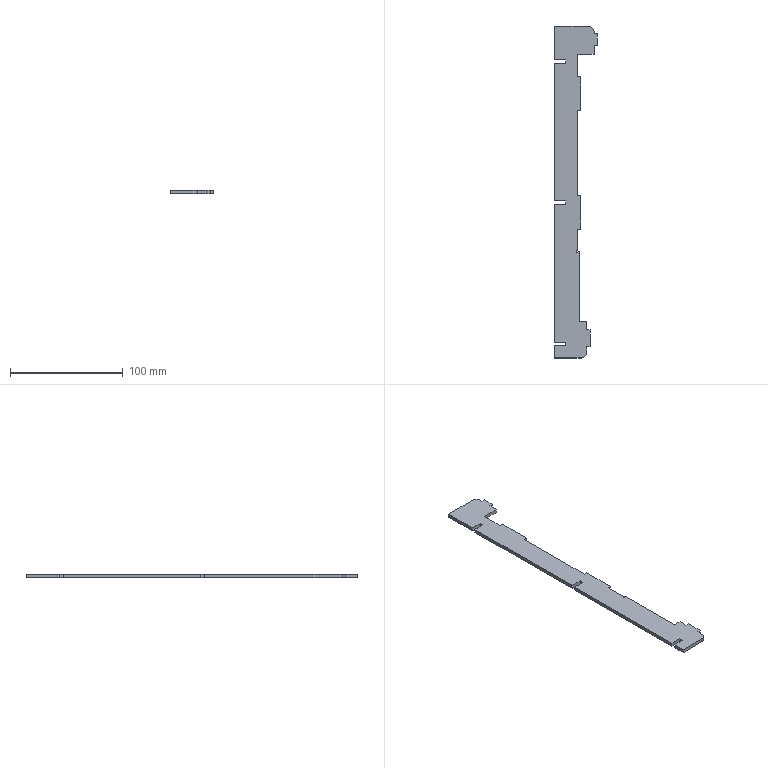Part | SolidWorks | features FlatPattern 1, SMBaseFlange 1, SheetMetal 1 | 1 solid | 46 faces | box 38 x 294.081 x 3.2 mm | volume 21708 mm3 | plane 40 | cylinder 6 | commonest cylinder face diameters 1 x2 1.5 x2 10 x2
STEP:
#1=CARTESIAN_POINT('',(397.65,-115.276,3.2));
#2=VERTEX_POINT('',#1);
#3=CARTESIAN_POINT('',(398.1,-114.588,3.2));
#4=VERTEX_POINT('',#3);
#5=CARTESIAN_POINT('',(398.4,-115.276,3.2));
#6=DIRECTION('',(0.,0.,-1.));
#7=DIRECTION('',(1.,0.,0.));
#8=AXIS2_PLACEMENT_3D('',#5,#6,#7);
#9=CIRCLE('',#8,0.75);
#10=EDGE_CURVE('',#2,#4,#9,.T.);
#11=ORIENTED_EDGE('',*,*,#10,.F.);
#12=CARTESIAN_POINT('',(397.65,-115.276,0.));
#13=VERTEX_POINT('',#12);
#14=CARTESIAN_POINT('',(397.65,-115.276,3.2));
#15=DIRECTION('',(0.,0.,-1.));
#16=VECTOR('',#15,1000.);
#17=LINE('',#14,#16);
#18=EDGE_CURVE('',#2,#13,#17,.T.);
#19=ORIENTED_EDGE('',*,*,#18,.T.);
#20=CARTESIAN_POINT('',(398.1,-114.588,0.));
#21=VERTEX_POINT('',#20);
#22=CARTESIAN_POINT('',(398.4,-115.276,0.));
#23=DIRECTION('',(0.,0.,-1.));
#24=DIRECTION('',(1.,0.,0.));
#25=AXIS2_PLACEMENT_3D('',#22,#23,#24);
#26=CIRCLE('',#25,0.75);
#27=EDGE_CURVE('',#13,#21,#26,.T.);
#28=ORIENTED_EDGE('',*,*,#27,.T.);
#29=CARTESIAN_POINT('',(398.1,-114.588,3.2));
#30=DIRECTION('',(0.,0.,-1.));
#31=VECTOR('',#30,1000.);
#32=LINE('',#29,#31);
#33=EDGE_CURVE('',#4,#21,#32,.T.);
#34=ORIENTED_EDGE('',*,*,#33,.F.);
#35=EDGE_LOOP('',(#11,#19,#28,#34));
#36=FACE_OUTER_BOUND('',#35,.T.);
#37=CARTESIAN_POINT('',(398.4,-115.276,3.2));
#38=DIRECTION('',(0.,0.,-1.));
#39=DIRECTION('',(-1.,0.,0.));
#40=AXIS2_PLACEMENT_3D('',#37,#38,#39);
#41=CYLINDRICAL_SURFACE('',#40,0.75);
#42=ADVANCED_FACE('',(#36),#41,.F.);
#43=CARTESIAN_POINT('',(413.4,59.724,0.));
#44=VERTEX_POINT('',#43);
#45=CARTESIAN_POINT('',(413.4,67.724,0.));
#46=VERTEX_POINT('',#45);
#47=CARTESIAN_POINT('',(413.4,59.724,0.));
#48=DIRECTION('',(0.,1.,0.));
#49=VECTOR('',#48,1000.);
#50=LINE('',#47,#49);
#51=EDGE_CURVE('',#44,#46,#50,.T.);
#52=ORIENTED_EDGE('',*,*,#51,.T.);
#53=CARTESIAN_POINT('',(413.4,67.724,3.2));
#54=VERTEX_POINT('',#53);
#55=CARTESIAN_POINT('',(413.4,67.724,3.2));
#56=DIRECTION('',(0.,0.,-1.));
#57=VECTOR('',#56,1000.);
#58=LINE('',#55,#57);
#59=EDGE_CURVE('',#54,#46,#58,.T.);
#60=ORIENTED_EDGE('',*,*,#59,.F.);
#61=CARTESIAN_POINT('',(413.4,59.724,3.2));
#62=VERTEX_POINT('',#61);
#63=CARTESIAN_POINT('',(413.4,59.724,3.2));
#64=DIRECTION('',(0.,1.,0.));
#65=VECTOR('',#64,1000.);
#66=LINE('',#63,#65);
#67=EDGE_CURVE('',#62,#54,#66,.T.);
#68=ORIENTED_EDGE('',*,*,#67,.F.);
#69=CARTESIAN_POINT('',(413.4,59.724,3.2));
#70=DIRECTION('',(0.,0.,-1.));
#71=VECTOR('',#70,1000.);
#72=LINE('',#69,#71);
#73=EDGE_CURVE('',#62,#44,#72,.T.);
#74=ORIENTED_EDGE('',*,*,#73,.T.);
#75=EDGE_LOOP('',(#52,#60,#68,#74));
#76=FACE_OUTER_BOUND('',#75,.T.);
#77=CARTESIAN_POINT('',(413.4,59.724,3.2));
#78=DIRECTION('',(-1.,0.,0.));
#79=DIRECTION('',(0.,-1.,0.));
#80=AXIS2_PLACEMENT_3D('',#77,#78,#79);
#81=PLANE('',#80);
#82=ADVANCED_FACE('',(#76),#81,.F.);
#83=CARTESIAN_POINT('',(416.4,67.724,0.));
#84=VERTEX_POINT('',#83);
#85=CARTESIAN_POINT('',(416.4,67.724,0.));
#86=DIRECTION('',(1.,0.,0.));
#87=VECTOR('',#86,1000.);
#88=LINE('',#85,#87);
#89=EDGE_CURVE('',#46,#84,#88,.T.);
#90=ORIENTED_EDGE('',*,*,#89,.T.);
#91=CARTESIAN_POINT('',(416.4,67.724,3.2));
#92=VERTEX_POINT('',#91);
#93=CARTESIAN_POINT('',(416.4,67.724,3.2));
#94=DIRECTION('',(0.,0.,-1.));
#95=VECTOR('',#94,1000.);
#96=LINE('',#93,#95);
#97=EDGE_CURVE('',#92,#84,#96,.T.);
#98=ORIENTED_EDGE('',*,*,#97,.F.);
#99=CARTESIAN_POINT('',(416.4,67.724,3.2));
#100=DIRECTION('',(1.,0.,0.));
#101=VECTOR('',#100,1000.);
#102=LINE('',#99,#101);
#103=EDGE_CURVE('',#54,#92,#102,.T.);
#104=ORIENTED_EDGE('',*,*,#103,.F.);
#105=ORIENTED_EDGE('',*,*,#59,.T.);
#106=EDGE_LOOP('',(#90,#98,#104,#105));
#107=FACE_OUTER_BOUND('',#106,.T.);
#108=CARTESIAN_POINT('',(416.4,67.724,3.2));
#109=DIRECTION('',(0.,1.,0.));
#110=DIRECTION('',(0.,0.,1.));
#111=AXIS2_PLACEMENT_3D('',#108,#109,#110);
#112=PLANE('',#111);
#113=ADVANCED_FACE('',(#107),#112,.F.);
#114=CARTESIAN_POINT('',(416.4,77.724,0.));
#115=VERTEX_POINT('',#114);
#116=CARTESIAN_POINT('',(416.4,77.724,0.));
#117=DIRECTION('',(0.,1.,0.));
#118=VECTOR('',#117,1000.);
#119=LINE('',#116,#118);
#120=EDGE_CURVE('',#84,#115,#119,.T.);
#121=ORIENTED_EDGE('',*,*,#120,.T.);
#122=CARTESIAN_POINT('',(416.4,77.724,3.2));
#123=VERTEX_POINT('',#122);
#124=CARTESIAN_POINT('',(416.4,77.724,3.2));
#125=DIRECTION('',(0.,0.,-1.));
#126=VECTOR('',#125,1000.);
#127=LINE('',#124,#126);
#128=EDGE_CURVE('',#123,#115,#127,.T.);
#129=ORIENTED_EDGE('',*,*,#128,.F.);
#130=CARTESIAN_POINT('',(416.4,77.724,3.2));
#131=DIRECTION('',(0.,1.,0.));
#132=VECTOR('',#131,1000.);
#133=LINE('',#130,#132);
#134=EDGE_CURVE('',#92,#123,#133,.T.);
#135=ORIENTED_EDGE('',*,*,#134,.F.);
#136=ORIENTED_EDGE('',*,*,#97,.T.);
#137=EDGE_LOOP('',(#121,#129,#135,#136));
#138=FACE_OUTER_BOUND('',#137,.T.);
#139=CARTESIAN_POINT('',(416.4,77.724,3.2));
#140=DIRECTION('',(-1.,0.,0.));
#141=DIRECTION('',(0.,0.,1.));
#142=AXIS2_PLACEMENT_3D('',#139,#140,#141);
#143=PLANE('',#142);
#144=ADVANCED_FACE('',(#138),#143,.F.);
#145=CARTESIAN_POINT('',(413.4,77.724,0.));
#146=VERTEX_POINT('',#145);
#147=CARTESIAN_POINT('',(413.4,77.724,0.));
#148=DIRECTION('',(-1.,0.,0.));
#149=VECTOR('',#148,1000.);
#150=LINE('',#147,#149);
#151=EDGE_CURVE('',#115,#146,#150,.T.);
#152=ORIENTED_EDGE('',*,*,#151,.T.);
#153=CARTESIAN_POINT('',(413.4,77.724,3.2));
#154=VERTEX_POINT('',#153);
#155=CARTESIAN_POINT('',(413.4,77.724,3.2));
#156=DIRECTION('',(0.,0.,-1.));
#157=VECTOR('',#156,1000.);
#158=LINE('',#155,#157);
#159=EDGE_CURVE('',#154,#146,#158,.T.);
#160=ORIENTED_EDGE('',*,*,#159,.F.);
#161=CARTESIAN_POINT('',(413.4,77.724,3.2));
#162=DIRECTION('',(-1.,0.,0.));
#163=VECTOR('',#162,1000.);
#164=LINE('',#161,#163);
#165=EDGE_CURVE('',#123,#154,#164,.T.);
#166=ORIENTED_EDGE('',*,*,#165,.F.);
#167=ORIENTED_EDGE('',*,*,#128,.T.);
#168=EDGE_LOOP('',(#152,#160,#166,#167));
#169=FACE_OUTER_BOUND('',#168,.T.);
#170=CARTESIAN_POINT('',(413.4,77.724,3.2));
#171=DIRECTION('',(0.,-1.,0.));
#172=DIRECTION('',(0.,0.,-1.));
#173=AXIS2_PLACEMENT_3D('',#170,#171,#172);
#174=PLANE('',#173);
#175=ADVANCED_FACE('',(#169),#174,.F.);
#176=CARTESIAN_POINT('',(413.4,79.724,0.));
#177=VERTEX_POINT('',#176);
#178=CARTESIAN_POINT('',(413.4,77.724,0.));
#179=DIRECTION('',(0.,1.,0.));
#180=VECTOR('',#179,1000.);
#181=LINE('',#178,#180);
#182=EDGE_CURVE('',#146,#177,#181,.T.);
#183=ORIENTED_EDGE('',*,*,#182,.T.);
#184=CARTESIAN_POINT('',(413.4,79.724,3.2));
#185=VERTEX_POINT('',#184);
#186=CARTESIAN_POINT('',(413.4,79.724,3.2));
#187=DIRECTION('',(0.,0.,-1.));
#188=VECTOR('',#187,1000.);
#189=LINE('',#186,#188);
#190=EDGE_CURVE('',#185,#177,#189,.T.);
#191=ORIENTED_EDGE('',*,*,#190,.F.);
#192=CARTESIAN_POINT('',(413.4,77.724,3.2));
#193=DIRECTION('',(0.,1.,0.));
#194=VECTOR('',#193,1000.);
#195=LINE('',#192,#194);
#196=EDGE_CURVE('',#154,#185,#195,.T.);
#197=ORIENTED_EDGE('',*,*,#196,.F.);
#198=ORIENTED_EDGE('',*,*,#159,.T.);
#199=EDGE_LOOP('',(#183,#191,#197,#198));
#200=FACE_OUTER_BOUND('',#199,.T.);
#201=CARTESIAN_POINT('',(413.4,77.724,3.2));
#202=DIRECTION('',(-1.,0.,0.));
#203=DIRECTION('',(0.,0.,1.));
#204=AXIS2_PLACEMENT_3D('',#201,#202,#203);
#205=PLANE('',#204);
#206=ADVANCED_FACE('',(#200),#205,.F.);
#207=CARTESIAN_POINT('',(408.4,84.724,0.));
#208=VERTEX_POINT('',#207);
#209=CARTESIAN_POINT('',(408.4,79.724,0.));
#210=DIRECTION('',(0.,0.,1.));
#211=DIRECTION('',(1.,0.,0.));
#212=AXIS2_PLACEMENT_3D('',#209,#210,#211);
#213=CIRCLE('',#212,5.);
#214=EDGE_CURVE('',#177,#208,#213,.T.);
#215=ORIENTED_EDGE('',*,*,#214,.T.);
#216=CARTESIAN_POINT('',(408.4,84.724,3.2));
#217=VERTEX_POINT('',#216);
#218=CARTESIAN_POINT('',(408.4,84.724,3.2));
#219=DIRECTION('',(0.,0.,-1.));
#220=VECTOR('',#219,1000.);
#221=LINE('',#218,#220);
#222=EDGE_CURVE('',#217,#208,#221,.T.);
#223=ORIENTED_EDGE('',*,*,#222,.F.);
#224=CARTESIAN_POINT('',(408.4,79.724,3.2));
#225=DIRECTION('',(0.,0.,1.));
#226=DIRECTION('',(1.,0.,0.));
#227=AXIS2_PLACEMENT_3D('',#224,#225,#226);
#228=CIRCLE('',#227,5.);
#229=EDGE_CURVE('',#185,#217,#228,.T.);
#230=ORIENTED_EDGE('',*,*,#229,.F.);
#231=ORIENTED_EDGE('',*,*,#190,.T.);
#232=EDGE_LOOP('',(#215,#223,#230,#231));
#233=FACE_OUTER_BOUND('',#232,.T.);
#234=CARTESIAN_POINT('',(408.4,79.724,3.2));
#235=DIRECTION('',(0.,0.,-1.));
#236=DIRECTION('',(-1.,0.,0.));
#237=AXIS2_PLACEMENT_3D('',#234,#235,#236);
#238=CYLINDRICAL_SURFACE('',#237,5.);
#239=ADVANCED_FACE('',(#233),#238,.T.);
#240=CARTESIAN_POINT('',(378.4,84.724,0.));
#241=VERTEX_POINT('',#240);
#242=CARTESIAN_POINT('',(408.4,84.724,0.));
#243=DIRECTION('',(-1.,0.,0.));
#244=VECTOR('',#243,1000.);
#245=LINE('',#242,#244);
#246=EDGE_CURVE('',#208,#241,#245,.T.);
#247=ORIENTED_EDGE('',*,*,#246,.T.);
#248=CARTESIAN_POINT('',(378.4,84.724,3.2));
#249=VERTEX_POINT('',#248);
#250=CARTESIAN_POINT('',(378.4,84.724,3.2));
#251=DIRECTION('',(0.,0.,-1.));
#252=VECTOR('',#251,1000.);
#253=LINE('',#250,#252);
#254=EDGE_CURVE('',#249,#241,#253,.T.);
#255=ORIENTED_EDGE('',*,*,#254,.F.);
#256=CARTESIAN_POINT('',(408.4,84.724,3.2));
#257=DIRECTION('',(-1.,0.,0.));
#258=VECTOR('',#257,1000.);
#259=LINE('',#256,#258);
#260=EDGE_CURVE('',#217,#249,#259,.T.);
#261=ORIENTED_EDGE('',*,*,#260,.F.);
#262=ORIENTED_EDGE('',*,*,#222,.T.);
#263=EDGE_LOOP('',(#247,#255,#261,#262));
#264=FACE_OUTER_BOUND('',#263,.T.);
#265=CARTESIAN_POINT('',(408.4,84.724,3.2));
#266=DIRECTION('',(0.,-1.,0.));
#267=DIRECTION('',(0.,0.,-1.));
#268=AXIS2_PLACEMENT_3D('',#265,#266,#267);
#269=PLANE('',#268);
#270=ADVANCED_FACE('',(#264),#269,.F.);
#271=CARTESIAN_POINT('',(378.4,54.724,0.));
#272=VERTEX_POINT('',#271);
#273=CARTESIAN_POINT('',(378.4,84.724,0.));
#274=DIRECTION('',(0.,-1.,0.));
#275=VECTOR('',#274,1000.);
#276=LINE('',#273,#275);
#277=EDGE_CURVE('',#241,#272,#276,.T.);
#278=ORIENTED_EDGE('',*,*,#277,.T.);
#279=CARTESIAN_POINT('',(378.4,54.724,3.2));
#280=VERTEX_POINT('',#279);
#281=CARTESIAN_POINT('',(378.4,54.724,3.2));
#282=DIRECTION('',(0.,0.,-1.));
#283=VECTOR('',#282,1000.);
#284=LINE('',#281,#283);
#285=EDGE_CURVE('',#280,#272,#284,.T.);
#286=ORIENTED_EDGE('',*,*,#285,.F.);
#287=CARTESIAN_POINT('',(378.4,84.724,3.2));
#288=DIRECTION('',(0.,-1.,0.));
#289=VECTOR('',#288,1000.);
#290=LINE('',#287,#289);
#291=EDGE_CURVE('',#249,#280,#290,.T.);
#292=ORIENTED_EDGE('',*,*,#291,.F.);
#293=ORIENTED_EDGE('',*,*,#254,.T.);
#294=EDGE_LOOP('',(#278,#286,#292,#293));
#295=FACE_OUTER_BOUND('',#294,.T.);
#296=CARTESIAN_POINT('',(378.4,84.724,3.2));
#297=DIRECTION('',(1.,0.,0.));
#298=DIRECTION('',(0.,0.,-1.));
#299=AXIS2_PLACEMENT_3D('',#296,#297,#298);
#300=PLANE('',#299);
#301=ADVANCED_FACE('',(#295),#300,.F.);
#302=CARTESIAN_POINT('',(388.4,54.724,0.));
#303=VERTEX_POINT('',#302);
#304=CARTESIAN_POINT('',(378.4,54.724,0.));
#305=DIRECTION('',(1.,0.000000036,0.));
#306=VECTOR('',#305,1000.);
#307=LINE('',#304,#306);
#308=EDGE_CURVE('',#272,#303,#307,.T.);
#309=ORIENTED_EDGE('',*,*,#308,.T.);
#310=CARTESIAN_POINT('',(388.4,54.724,3.2));
#311=VERTEX_POINT('',#310);
#312=CARTESIAN_POINT('',(388.4,54.724,3.2));
#313=DIRECTION('',(0.,0.,-1.));
#314=VECTOR('',#313,1000.);
#315=LINE('',#312,#314);
#316=EDGE_CURVE('',#311,#303,#315,.T.);
#317=ORIENTED_EDGE('',*,*,#316,.F.);
#318=CARTESIAN_POINT('',(378.4,54.724,3.2));
#319=DIRECTION('',(1.,0.000000036,0.));
#320=VECTOR('',#319,1000.);
#321=LINE('',#318,#320);
#322=EDGE_CURVE('',#280,#311,#321,.T.);
#323=ORIENTED_EDGE('',*,*,#322,.F.);
#324=ORIENTED_EDGE('',*,*,#285,.T.);
#325=EDGE_LOOP('',(#309,#317,#323,#324));
#326=FACE_OUTER_BOUND('',#325,.T.);
#327=CARTESIAN_POINT('',(378.4,54.724,3.2));
#328=DIRECTION('',(-0.000000036,1.,0.));
#329=DIRECTION('',(-1.,-0.000000036,0.));
#330=AXIS2_PLACEMENT_3D('',#327,#328,#329);
#331=PLANE('',#330);
#332=ADVANCED_FACE('',(#326),#331,.F.);
#333=CARTESIAN_POINT('',(388.4,51.524,0.));
#334=VERTEX_POINT('',#333);
#335=CARTESIAN_POINT('',(388.4,54.724,0.));
#336=DIRECTION('',(0.000000036,-1.,0.));
#337=VECTOR('',#336,1000.);
#338=LINE('',#335,#337);
#339=EDGE_CURVE('',#303,#334,#338,.T.);
#340=ORIENTED_EDGE('',*,*,#339,.T.);
#341=CARTESIAN_POINT('',(388.4,51.524,3.2));
#342=VERTEX_POINT('',#341);
#343=CARTESIAN_POINT('',(388.4,51.524,3.2));
#344=DIRECTION('',(0.,0.,-1.));
#345=VECTOR('',#344,1000.);
#346=LINE('',#343,#345);
#347=EDGE_CURVE('',#342,#334,#346,.T.);
#348=ORIENTED_EDGE('',*,*,#347,.F.);
#349=CARTESIAN_POINT('',(388.4,54.724,3.2));
#350=DIRECTION('',(0.000000036,-1.,0.));
#351=VECTOR('',#350,1000.);
#352=LINE('',#349,#351);
#353=EDGE_CURVE('',#311,#342,#352,.T.);
#354=ORIENTED_EDGE('',*,*,#353,.F.);
#355=ORIENTED_EDGE('',*,*,#316,.T.);
#356=EDGE_LOOP('',(#340,#348,#354,#355));
#357=FACE_OUTER_BOUND('',#356,.T.);
#358=CARTESIAN_POINT('',(388.4,54.724,3.2));
#359=DIRECTION('',(1.,0.000000036,0.));
#360=DIRECTION('',(-0.000000036,1.,0.));
#361=AXIS2_PLACEMENT_3D('',#358,#359,#360);
#362=PLANE('',#361);
#363=ADVANCED_FACE('',(#357),#362,.F.);
#364=CARTESIAN_POINT('',(378.4,51.524,0.));
#365=VERTEX_POINT('',#364);
#366=CARTESIAN_POINT('',(388.4,51.524,0.));
#367=DIRECTION('',(-1.,-0.000000036,0.));
#368=VECTOR('',#367,1000.);
#369=LINE('',#366,#368);
#370=EDGE_CURVE('',#334,#365,#369,.T.);
#371=ORIENTED_EDGE('',*,*,#370,.T.);
#372=CARTESIAN_POINT('',(378.4,51.524,3.2));
#373=VERTEX_POINT('',#372);
#374=CARTESIAN_POINT('',(378.4,51.524,3.2));
#375=DIRECTION('',(0.,0.,-1.));
#376=VECTOR('',#375,1000.);
#377=LINE('',#374,#376);
#378=EDGE_CURVE('',#373,#365,#377,.T.);
#379=ORIENTED_EDGE('',*,*,#378,.F.);
#380=CARTESIAN_POINT('',(388.4,51.524,3.2));
#381=DIRECTION('',(-1.,-0.000000036,0.));
#382=VECTOR('',#381,1000.);
#383=LINE('',#380,#382);
#384=EDGE_CURVE('',#342,#373,#383,.T.);
#385=ORIENTED_EDGE('',*,*,#384,.F.);
#386=ORIENTED_EDGE('',*,*,#347,.T.);
#387=EDGE_LOOP('',(#371,#379,#385,#386));
#388=FACE_OUTER_BOUND('',#387,.T.);
#389=CARTESIAN_POINT('',(388.4,51.524,3.2));
#390=DIRECTION('',(0.000000036,-1.,0.));
#391=DIRECTION('',(1.,0.000000036,0.));
#392=AXIS2_PLACEMENT_3D('',#389,#390,#391);
#393=PLANE('',#392);
#394=ADVANCED_FACE('',(#388),#393,.F.);
#395=CARTESIAN_POINT('',(378.4,-70.276,0.));
#396=VERTEX_POINT('',#395);
#397=CARTESIAN_POINT('',(378.4,51.524,0.));
#398=DIRECTION('',(-0.000000001,-1.,0.));
#399=VECTOR('',#398,1000.);
#400=LINE('',#397,#399);
#401=EDGE_CURVE('',#365,#396,#400,.T.);
#402=ORIENTED_EDGE('',*,*,#401,.T.);
#403=CARTESIAN_POINT('',(378.4,-70.276,3.2));
#404=VERTEX_POINT('',#403);
#405=CARTESIAN_POINT('',(378.4,-70.276,3.2));
#406=DIRECTION('',(0.,0.,-1.));
#407=VECTOR('',#406,1000.);
#408=LINE('',#405,#407);
#409=EDGE_CURVE('',#404,#396,#408,.T.);
#410=ORIENTED_EDGE('',*,*,#409,.F.);
#411=CARTESIAN_POINT('',(378.4,51.524,3.2));
#412=DIRECTION('',(-0.000000001,-1.,0.));
#413=VECTOR('',#412,1000.);
#414=LINE('',#411,#413);
#415=EDGE_CURVE('',#373,#404,#414,.T.);
#416=ORIENTED_EDGE('',*,*,#415,.F.);
#417=ORIENTED_EDGE('',*,*,#378,.T.);
#418=EDGE_LOOP('',(#402,#410,#416,#417));
#419=FACE_OUTER_BOUND('',#418,.T.);
#420=CARTESIAN_POINT('',(378.4,51.524,3.2));
#421=DIRECTION('',(1.,-0.000000001,0.));
#422=DIRECTION('',(0.000000001,1.,0.));
#423=AXIS2_PLACEMENT_3D('',#420,#421,#422);
#424=PLANE('',#423);
#425=ADVANCED_FACE('',(#419),#424,.F.);
#426=CARTESIAN_POINT('',(388.4,-70.276,0.));
#427=VERTEX_POINT('',#426);
#428=CARTESIAN_POINT('',(378.4,-70.276,0.));
#429=DIRECTION('',(1.,0.000000036,0.));
#430=VECTOR('',#429,1000.);
#431=LINE('',#428,#430);
#432=EDGE_CURVE('',#396,#427,#431,.T.);
#433=ORIENTED_EDGE('',*,*,#432,.T.);
#434=CARTESIAN_POINT('',(388.4,-70.276,3.2));
#435=VERTEX_POINT('',#434);
#436=CARTESIAN_POINT('',(388.4,-70.276,3.2));
#437=DIRECTION('',(0.,0.,-1.));
#438=VECTOR('',#437,1000.);
#439=LINE('',#436,#438);
#440=EDGE_CURVE('',#435,#427,#439,.T.);
#441=ORIENTED_EDGE('',*,*,#440,.F.);
#442=CARTESIAN_POINT('',(378.4,-70.276,3.2));
#443=DIRECTION('',(1.,0.000000036,0.));
#444=VECTOR('',#443,1000.);
#445=LINE('',#442,#444);
#446=EDGE_CURVE('',#404,#435,#445,.T.);
#447=ORIENTED_EDGE('',*,*,#446,.F.);
#448=ORIENTED_EDGE('',*,*,#409,.T.);
#449=EDGE_LOOP('',(#433,#441,#447,#448));
#450=FACE_OUTER_BOUND('',#449,.T.);
#451=CARTESIAN_POINT('',(378.4,-70.276,3.2));
#452=DIRECTION('',(-0.000000036,1.,0.));
#453=DIRECTION('',(-1.,-0.000000036,0.));
#454=AXIS2_PLACEMENT_3D('',#451,#452,#453);
#455=PLANE('',#454);
#456=ADVANCED_FACE('',(#450),#455,.F.);
#457=CARTESIAN_POINT('',(388.4,-73.476,0.));
#458=VERTEX_POINT('',#457);
#459=CARTESIAN_POINT('',(388.4,-70.276,0.));
#460=DIRECTION('',(0.000000036,-1.,0.));
#461=VECTOR('',#460,1000.);
#462=LINE('',#459,#461);
#463=EDGE_CURVE('',#427,#458,#462,.T.);
#464=ORIENTED_EDGE('',*,*,#463,.T.);
#465=CARTESIAN_POINT('',(388.4,-73.476,3.2));
#466=VERTEX_POINT('',#465);
#467=CARTESIAN_POINT('',(388.4,-73.476,3.2));
#468=DIRECTION('',(0.,0.,-1.));
#469=VECTOR('',#468,1000.);
#470=LINE('',#467,#469);
#471=EDGE_CURVE('',#466,#458,#470,.T.);
#472=ORIENTED_EDGE('',*,*,#471,.F.);
#473=CARTESIAN_POINT('',(388.4,-70.276,3.2));
#474=DIRECTION('',(0.000000036,-1.,0.));
#475=VECTOR('',#474,1000.);
#476=LINE('',#473,#475);
#477=EDGE_CURVE('',#435,#466,#476,.T.);
#478=ORIENTED_EDGE('',*,*,#477,.F.);
#479=ORIENTED_EDGE('',*,*,#440,.T.);
#480=EDGE_LOOP('',(#464,#472,#478,#479));
#481=FACE_OUTER_BOUND('',#480,.T.);
#482=CARTESIAN_POINT('',(388.4,-70.276,3.2));
#483=DIRECTION('',(1.,0.000000036,0.));
#484=DIRECTION('',(-0.000000036,1.,0.));
#485=AXIS2_PLACEMENT_3D('',#482,#483,#484);
#486=PLANE('',#485);
#487=ADVANCED_FACE('',(#481),#486,.F.);
#488=CARTESIAN_POINT('',(378.4,-73.476,0.));
#489=VERTEX_POINT('',#488);
#490=CARTESIAN_POINT('',(388.4,-73.476,0.));
#491=DIRECTION('',(-1.,-0.000000036,0.));
#492=VECTOR('',#491,1000.);
#493=LINE('',#490,#492);
#494=EDGE_CURVE('',#458,#489,#493,.T.);
#495=ORIENTED_EDGE('',*,*,#494,.T.);
#496=CARTESIAN_POINT('',(378.4,-73.476,3.2));
#497=VERTEX_POINT('',#496);
#498=CARTESIAN_POINT('',(378.4,-73.476,3.2));
#499=DIRECTION('',(0.,0.,-1.));
#500=VECTOR('',#499,1000.);
#501=LINE('',#498,#500);
#502=EDGE_CURVE('',#497,#489,#501,.T.);
#503=ORIENTED_EDGE('',*,*,#502,.F.);
#504=CARTESIAN_POINT('',(388.4,-73.476,3.2));
#505=DIRECTION('',(-1.,-0.000000036,0.));
#506=VECTOR('',#505,1000.);
#507=LINE('',#504,#506);
#508=EDGE_CURVE('',#466,#497,#507,.T.);
#509=ORIENTED_EDGE('',*,*,#508,.F.);
#510=ORIENTED_EDGE('',*,*,#471,.T.);
#511=EDGE_LOOP('',(#495,#503,#509,#510));
#512=FACE_OUTER_BOUND('',#511,.T.);
#513=CARTESIAN_POINT('',(388.4,-73.476,3.2));
#514=DIRECTION('',(0.000000036,-1.,0.));
#515=DIRECTION('',(1.,0.000000036,0.));
#516=AXIS2_PLACEMENT_3D('',#513,#514,#515);
#517=PLANE('',#516);
#518=ADVANCED_FACE('',(#512),#517,.F.);
#519=CARTESIAN_POINT('',(378.4,-195.276,0.));
#520=VERTEX_POINT('',#519);
#521=CARTESIAN_POINT('',(378.4,-73.476,0.));
#522=DIRECTION('',(-0.000000001,-1.,0.));
#523=VECTOR('',#522,1000.);
#524=LINE('',#521,#523);
#525=EDGE_CURVE('',#489,#520,#524,.T.);
#526=ORIENTED_EDGE('',*,*,#525,.T.);
#527=CARTESIAN_POINT('',(378.4,-195.276,3.2));
#528=VERTEX_POINT('',#527);
#529=CARTESIAN_POINT('',(378.4,-195.276,3.2));
#530=DIRECTION('',(0.,0.,-1.));
#531=VECTOR('',#530,1000.);
#532=LINE('',#529,#531);
#533=EDGE_CURVE('',#528,#520,#532,.T.);
#534=ORIENTED_EDGE('',*,*,#533,.F.);
#535=CARTESIAN_POINT('',(378.4,-73.476,3.2));
#536=DIRECTION('',(-0.000000001,-1.,0.));
#537=VECTOR('',#536,1000.);
#538=LINE('',#535,#537);
#539=EDGE_CURVE('',#497,#528,#538,.T.);
#540=ORIENTED_EDGE('',*,*,#539,.F.);
#541=ORIENTED_EDGE('',*,*,#502,.T.);
#542=EDGE_LOOP('',(#526,#534,#540,#541));
#543=FACE_OUTER_BOUND('',#542,.T.);
#544=CARTESIAN_POINT('',(378.4,-73.476,3.2));
#545=DIRECTION('',(1.,-0.000000001,0.));
#546=DIRECTION('',(0.000000001,1.,0.));
#547=AXIS2_PLACEMENT_3D('',#544,#545,#546);
#548=PLANE('',#547);
#549=ADVANCED_FACE('',(#543),#548,.F.);
#550=CARTESIAN_POINT('',(388.4,-195.276,0.));
#551=VERTEX_POINT('',#550);
#552=CARTESIAN_POINT('',(388.4,-195.276,0.));
#553=DIRECTION('',(1.,0.000000072,0.));
#554=VECTOR('',#553,1000.);
#555=LINE('',#552,#554);
#556=EDGE_CURVE('',#520,#551,#555,.T.);
#557=ORIENTED_EDGE('',*,*,#556,.T.);
#558=CARTESIAN_POINT('',(388.4,-195.276,3.2));
#559=VERTEX_POINT('',#558);
#560=CARTESIAN_POINT('',(388.4,-195.276,3.2));
#561=DIRECTION('',(0.,0.,-1.));
#562=VECTOR('',#561,1000.);
#563=LINE('',#560,#562);
#564=EDGE_CURVE('',#559,#551,#563,.T.);
#565=ORIENTED_EDGE('',*,*,#564,.F.);
#566=CARTESIAN_POINT('',(388.4,-195.276,3.2));
#567=DIRECTION('',(1.,0.000000072,0.));
#568=VECTOR('',#567,1000.);
#569=LINE('',#566,#568);
#570=EDGE_CURVE('',#528,#559,#569,.T.);
#571=ORIENTED_EDGE('',*,*,#570,.F.);
#572=ORIENTED_EDGE('',*,*,#533,.T.);
#573=EDGE_LOOP('',(#557,#565,#571,#572));
#574=FACE_OUTER_BOUND('',#573,.T.);
#575=CARTESIAN_POINT('',(388.4,-195.276,3.2));
#576=DIRECTION('',(-0.000000072,1.,0.));
#577=DIRECTION('',(-1.,-0.000000072,0.));
#578=AXIS2_PLACEMENT_3D('',#575,#576,#577);
#579=PLANE('',#578);
#580=ADVANCED_FACE('',(#574),#579,.F.);
#581=CARTESIAN_POINT('',(388.4,-198.476,0.));
#582=VERTEX_POINT('',#581);
#583=CARTESIAN_POINT('',(388.4,-198.476,0.));
#584=DIRECTION('',(0.,-1.,0.));
#585=VECTOR('',#584,1000.);
#586=LINE('',#583,#585);
#587=EDGE_CURVE('',#551,#582,#586,.T.);
#588=ORIENTED_EDGE('',*,*,#587,.T.);
#589=CARTESIAN_POINT('',(388.4,-198.476,3.2));
#590=VERTEX_POINT('',#589);
#591=CARTESIAN_POINT('',(388.4,-198.476,3.2));
#592=DIRECTION('',(0.,0.,-1.));
#593=VECTOR('',#592,1000.);
#594=LINE('',#591,#593);
#595=EDGE_CURVE('',#590,#582,#594,.T.);
#596=ORIENTED_EDGE('',*,*,#595,.F.);
#597=CARTESIAN_POINT('',(388.4,-198.476,3.2));
#598=DIRECTION('',(0.,-1.,0.));
#599=VECTOR('',#598,1000.);
#600=LINE('',#597,#599);
#601=EDGE_CURVE('',#559,#590,#600,.T.);
#602=ORIENTED_EDGE('',*,*,#601,.F.);
#603=ORIENTED_EDGE('',*,*,#564,.T.);
#604=EDGE_LOOP('',(#588,#596,#602,#603));
#605=FACE_OUTER_BOUND('',#604,.T.);
#606=CARTESIAN_POINT('',(388.4,-198.476,3.2));
#607=DIRECTION('',(1.,0.,0.));
#608=DIRECTION('',(0.,0.,-1.));
#609=AXIS2_PLACEMENT_3D('',#606,#607,#608);
#610=PLANE('',#609);
#611=ADVANCED_FACE('',(#605),#610,.F.);
#612=CARTESIAN_POINT('',(378.4,-198.476,0.));
#613=VERTEX_POINT('',#612);
#614=CARTESIAN_POINT('',(378.4,-198.476,0.));
#615=DIRECTION('',(-1.,-0.000000072,0.));
#616=VECTOR('',#615,1000.);
#617=LINE('',#614,#616);
#618=EDGE_CURVE('',#582,#613,#617,.T.);
#619=ORIENTED_EDGE('',*,*,#618,.T.);
#620=CARTESIAN_POINT('',(378.4,-198.476,3.2));
#621=VERTEX_POINT('',#620);
#622=CARTESIAN_POINT('',(378.4,-198.476,3.2));
#623=DIRECTION('',(0.,0.,-1.));
#624=VECTOR('',#623,1000.);
#625=LINE('',#622,#624);
#626=EDGE_CURVE('',#621,#613,#625,.T.);
#627=ORIENTED_EDGE('',*,*,#626,.F.);
#628=CARTESIAN_POINT('',(378.4,-198.476,3.2));
#629=DIRECTION('',(-1.,-0.000000072,0.));
#630=VECTOR('',#629,1000.);
#631=LINE('',#628,#630);
#632=EDGE_CURVE('',#590,#621,#631,.T.);
#633=ORIENTED_EDGE('',*,*,#632,.F.);
#634=ORIENTED_EDGE('',*,*,#595,.T.);
#635=EDGE_LOOP('',(#619,#627,#633,#634));
#636=FACE_OUTER_BOUND('',#635,.T.);
#637=CARTESIAN_POINT('',(378.4,-198.476,3.2));
#638=DIRECTION('',(0.000000072,-1.,0.));
#639=DIRECTION('',(1.,0.000000072,0.));
#640=AXIS2_PLACEMENT_3D('',#637,#638,#639);
#641=PLANE('',#640);
#642=ADVANCED_FACE('',(#636),#641,.F.);
#643=CARTESIAN_POINT('',(378.4,-209.357,0.));
#644=VERTEX_POINT('',#643);
#645=CARTESIAN_POINT('',(378.4,-198.476,0.));
#646=DIRECTION('',(-0.000000011,-1.,0.));
#647=VECTOR('',#646,1000.);
#648=LINE('',#645,#647);
#649=EDGE_CURVE('',#613,#644,#648,.T.);
#650=ORIENTED_EDGE('',*,*,#649,.T.);
#651=CARTESIAN_POINT('',(378.4,-209.357,3.2));
#652=VERTEX_POINT('',#651);
#653=CARTESIAN_POINT('',(378.4,-209.357,3.2));
#654=DIRECTION('',(0.,0.,-1.));
#655=VECTOR('',#654,1000.);
#656=LINE('',#653,#655);
#657=EDGE_CURVE('',#652,#644,#656,.T.);
#658=ORIENTED_EDGE('',*,*,#657,.F.);
#659=CARTESIAN_POINT('',(378.4,-198.476,3.2));
#660=DIRECTION('',(-0.000000011,-1.,0.));
#661=VECTOR('',#660,1000.);
#662=LINE('',#659,#661);
#663=EDGE_CURVE('',#621,#652,#662,.T.);
#664=ORIENTED_EDGE('',*,*,#663,.F.);
#665=ORIENTED_EDGE('',*,*,#626,.T.);
#666=EDGE_LOOP('',(#650,#658,#664,#665));
#667=FACE_OUTER_BOUND('',#666,.T.);
#668=CARTESIAN_POINT('',(378.4,-198.476,3.2));
#669=DIRECTION('',(1.,-0.000000011,0.));
#670=DIRECTION('',(0.000000011,1.,0.));
#671=AXIS2_PLACEMENT_3D('',#668,#669,#670);
#672=PLANE('',#671);
#673=ADVANCED_FACE('',(#667),#672,.F.);
#674=CARTESIAN_POINT('',(401.9,-209.357,0.));
#675=VERTEX_POINT('',#674);
#676=CARTESIAN_POINT('',(378.4,-209.357,0.));
#677=DIRECTION('',(1.,0.,0.));
#678=VECTOR('',#677,1000.);
#679=LINE('',#676,#678);
#680=EDGE_CURVE('',#644,#675,#679,.T.);
#681=ORIENTED_EDGE('',*,*,#680,.T.);
#682=CARTESIAN_POINT('',(401.9,-209.357,3.2));
#683=VERTEX_POINT('',#682);
#684=CARTESIAN_POINT('',(401.9,-209.357,3.2));
#685=DIRECTION('',(0.,0.,-1.));
#686=VECTOR('',#685,1000.);
#687=LINE('',#684,#686);
#688=EDGE_CURVE('',#683,#675,#687,.T.);
#689=ORIENTED_EDGE('',*,*,#688,.F.);
#690=CARTESIAN_POINT('',(378.4,-209.357,3.2));
#691=DIRECTION('',(1.,0.,0.));
#692=VECTOR('',#691,1000.);
#693=LINE('',#690,#692);
#694=EDGE_CURVE('',#652,#683,#693,.T.);
#695=ORIENTED_EDGE('',*,*,#694,.F.);
#696=ORIENTED_EDGE('',*,*,#657,.T.);
#697=EDGE_LOOP('',(#681,#689,#695,#696));
#698=FACE_OUTER_BOUND('',#697,.T.);
#699=CARTESIAN_POINT('',(378.4,-209.357,3.2));
#700=DIRECTION('',(0.,1.,0.));
#701=DIRECTION('',(-1.,0.,0.));
#702=AXIS2_PLACEMENT_3D('',#699,#700,#701);
#703=PLANE('',#702);
#704=ADVANCED_FACE('',(#698),#703,.F.);
#705=CARTESIAN_POINT('',(406.9,-204.357,0.));
#706=VERTEX_POINT('',#705);
#707=CARTESIAN_POINT('',(401.9,-204.357,0.));
#708=DIRECTION('',(0.,0.,1.));
#709=DIRECTION('',(1.,0.,0.));
#710=AXIS2_PLACEMENT_3D('',#707,#708,#709);
#711=CIRCLE('',#710,5.);
#712=EDGE_CURVE('',#675,#706,#711,.T.);
#713=ORIENTED_EDGE('',*,*,#712,.T.);
#714=CARTESIAN_POINT('',(406.9,-204.357,3.2));
#715=VERTEX_POINT('',#714);
#716=CARTESIAN_POINT('',(406.9,-204.357,3.2));
#717=DIRECTION('',(0.,0.,-1.));
#718=VECTOR('',#717,1000.);
#719=LINE('',#716,#718);
#720=EDGE_CURVE('',#715,#706,#719,.T.);
#721=ORIENTED_EDGE('',*,*,#720,.F.);
#722=CARTESIAN_POINT('',(401.9,-204.357,3.2));
#723=DIRECTION('',(0.,0.,1.));
#724=DIRECTION('',(1.,0.,0.));
#725=AXIS2_PLACEMENT_3D('',#722,#723,#724);
#726=CIRCLE('',#725,5.);
#727=EDGE_CURVE('',#683,#715,#726,.T.);
#728=ORIENTED_EDGE('',*,*,#727,.F.);
#729=ORIENTED_EDGE('',*,*,#688,.T.);
#730=EDGE_LOOP('',(#713,#721,#728,#729));
#731=FACE_OUTER_BOUND('',#730,.T.);
#732=CARTESIAN_POINT('',(401.9,-204.357,3.2));
#733=DIRECTION('',(0.,0.,-1.));
#734=DIRECTION('',(-1.,0.,0.));
#735=AXIS2_PLACEMENT_3D('',#732,#733,#734);
#736=CYLINDRICAL_SURFACE('',#735,5.);
#737=ADVANCED_FACE('',(#731),#736,.T.);
#738=CARTESIAN_POINT('',(406.9,-199.357,0.));
#739=VERTEX_POINT('',#738);
#740=CARTESIAN_POINT('',(406.9,-204.357,0.));
#741=DIRECTION('',(0.,1.,0.));
#742=VECTOR('',#741,1000.);
#743=LINE('',#740,#742);
#744=EDGE_CURVE('',#706,#739,#743,.T.);
#745=ORIENTED_EDGE('',*,*,#744,.T.);
#746=CARTESIAN_POINT('',(406.9,-199.357,3.2));
#747=VERTEX_POINT('',#746);
#748=CARTESIAN_POINT('',(406.9,-199.357,3.2));
#749=DIRECTION('',(0.,0.,-1.));
#750=VECTOR('',#749,1000.);
#751=LINE('',#748,#750);
#752=EDGE_CURVE('',#747,#739,#751,.T.);
#753=ORIENTED_EDGE('',*,*,#752,.F.);
#754=CARTESIAN_POINT('',(406.9,-204.357,3.2));
#755=DIRECTION('',(0.,1.,0.));
#756=VECTOR('',#755,1000.);
#757=LINE('',#754,#756);
#758=EDGE_CURVE('',#715,#747,#757,.T.);
#759=ORIENTED_EDGE('',*,*,#758,.F.);
#760=ORIENTED_EDGE('',*,*,#720,.T.);
#761=EDGE_LOOP('',(#745,#753,#759,#760));
#762=FACE_OUTER_BOUND('',#761,.T.);
#763=CARTESIAN_POINT('',(406.9,-204.357,3.2));
#764=DIRECTION('',(-1.,0.,0.));
#765=DIRECTION('',(0.,0.,1.));
#766=AXIS2_PLACEMENT_3D('',#763,#764,#765);
#767=PLANE('',#766);
#768=ADVANCED_FACE('',(#762),#767,.F.);
#769=CARTESIAN_POINT('',(409.9,-199.357,0.));
#770=VERTEX_POINT('',#769);
#771=CARTESIAN_POINT('',(406.9,-199.357,0.));
#772=DIRECTION('',(1.,0.,0.));
#773=VECTOR('',#772,1000.);
#774=LINE('',#771,#773);
#775=EDGE_CURVE('',#739,#770,#774,.T.);
#776=ORIENTED_EDGE('',*,*,#775,.T.);
#777=CARTESIAN_POINT('',(409.9,-199.357,3.2));
#778=VERTEX_POINT('',#777);
#779=CARTESIAN_POINT('',(409.9,-199.357,3.2));
#780=DIRECTION('',(0.,0.,-1.));
#781=VECTOR('',#780,1000.);
#782=LINE('',#779,#781);
#783=EDGE_CURVE('',#778,#770,#782,.T.);
#784=ORIENTED_EDGE('',*,*,#783,.F.);
#785=CARTESIAN_POINT('',(406.9,-199.357,3.2));
#786=DIRECTION('',(1.,0.,0.));
#787=VECTOR('',#786,1000.);
#788=LINE('',#785,#787);
#789=EDGE_CURVE('',#747,#778,#788,.T.);
#790=ORIENTED_EDGE('',*,*,#789,.F.);
#791=ORIENTED_EDGE('',*,*,#752,.T.);
#792=EDGE_LOOP('',(#776,#784,#790,#791));
#793=FACE_OUTER_BOUND('',#792,.T.);
#794=CARTESIAN_POINT('',(406.9,-199.357,3.2));
#795=DIRECTION('',(0.,1.,0.));
#796=DIRECTION('',(0.,0.,1.));
#797=AXIS2_PLACEMENT_3D('',#794,#795,#796);
#798=PLANE('',#797);
#799=ADVANCED_FACE('',(#793),#798,.F.);
#800=CARTESIAN_POINT('',(409.9,-184.357,0.));
#801=VERTEX_POINT('',#800);
#802=CARTESIAN_POINT('',(409.9,-199.357,0.));
#803=DIRECTION('',(0.,1.,0.));
#804=VECTOR('',#803,1000.);
#805=LINE('',#802,#804);
#806=EDGE_CURVE('',#770,#801,#805,.T.);
#807=ORIENTED_EDGE('',*,*,#806,.T.);
#808=CARTESIAN_POINT('',(409.9,-184.357,3.2));
#809=VERTEX_POINT('',#808);
#810=CARTESIAN_POINT('',(409.9,-184.357,3.2));
#811=DIRECTION('',(0.,0.,-1.));
#812=VECTOR('',#811,1000.);
#813=LINE('',#810,#812);
#814=EDGE_CURVE('',#809,#801,#813,.T.);
#815=ORIENTED_EDGE('',*,*,#814,.F.);
#816=CARTESIAN_POINT('',(409.9,-199.357,3.2));
#817=DIRECTION('',(0.,1.,0.));
#818=VECTOR('',#817,1000.);
#819=LINE('',#816,#818);
#820=EDGE_CURVE('',#778,#809,#819,.T.);
#821=ORIENTED_EDGE('',*,*,#820,.F.);
#822=ORIENTED_EDGE('',*,*,#783,.T.);
#823=EDGE_LOOP('',(#807,#815,#821,#822));
#824=FACE_OUTER_BOUND('',#823,.T.);
#825=CARTESIAN_POINT('',(409.9,-199.357,3.2));
#826=DIRECTION('',(-1.,0.,0.));
#827=DIRECTION('',(0.,0.,1.));
#828=AXIS2_PLACEMENT_3D('',#825,#826,#827);
#829=PLANE('',#828);
#830=ADVANCED_FACE('',(#824),#829,.F.);
#831=CARTESIAN_POINT('',(406.9,-184.357,0.));
#832=VERTEX_POINT('',#831);
#833=CARTESIAN_POINT('',(409.9,-184.357,0.));
#834=DIRECTION('',(-1.,0.,0.));
#835=VECTOR('',#834,1000.);
#836=LINE('',#833,#835);
#837=EDGE_CURVE('',#801,#832,#836,.T.);
#838=ORIENTED_EDGE('',*,*,#837,.T.);
#839=CARTESIAN_POINT('',(406.9,-184.357,3.2));
#840=VERTEX_POINT('',#839);
#841=CARTESIAN_POINT('',(406.9,-184.357,3.2));
#842=DIRECTION('',(0.,0.,-1.));
#843=VECTOR('',#842,1000.);
#844=LINE('',#841,#843);
#845=EDGE_CURVE('',#840,#832,#844,.T.);
#846=ORIENTED_EDGE('',*,*,#845,.F.);
#847=CARTESIAN_POINT('',(409.9,-184.357,3.2));
#848=DIRECTION('',(-1.,0.,0.));
#849=VECTOR('',#848,1000.);
#850=LINE('',#847,#849);
#851=EDGE_CURVE('',#809,#840,#850,.T.);
#852=ORIENTED_EDGE('',*,*,#851,.F.);
#853=ORIENTED_EDGE('',*,*,#814,.T.);
#854=EDGE_LOOP('',(#838,#846,#852,#853));
#855=FACE_OUTER_BOUND('',#854,.T.);
#856=CARTESIAN_POINT('',(409.9,-184.357,3.2));
#857=DIRECTION('',(0.,-1.,0.));
#858=DIRECTION('',(1.,0.,0.));
#859=AXIS2_PLACEMENT_3D('',#856,#857,#858);
#860=PLANE('',#859);
#861=ADVANCED_FACE('',(#855),#860,.F.);
#862=CARTESIAN_POINT('',(406.9,-176.957,0.));
#863=VERTEX_POINT('',#862);
#864=CARTESIAN_POINT('',(406.9,-184.357,0.));
#865=DIRECTION('',(0.,1.,0.));
#866=VECTOR('',#865,1000.);
#867=LINE('',#864,#866);
#868=EDGE_CURVE('',#832,#863,#867,.T.);
#869=ORIENTED_EDGE('',*,*,#868,.T.);
#870=CARTESIAN_POINT('',(406.9,-176.957,3.2));
#871=VERTEX_POINT('',#870);
#872=CARTESIAN_POINT('',(406.9,-176.957,3.2));
#873=DIRECTION('',(0.,0.,-1.));
#874=VECTOR('',#873,1000.);
#875=LINE('',#872,#874);
#876=EDGE_CURVE('',#871,#863,#875,.T.);
#877=ORIENTED_EDGE('',*,*,#876,.F.);
#878=CARTESIAN_POINT('',(406.9,-184.357,3.2));
#879=DIRECTION('',(0.,1.,0.));
#880=VECTOR('',#879,1000.);
#881=LINE('',#878,#880);
#882=EDGE_CURVE('',#840,#871,#881,.T.);
#883=ORIENTED_EDGE('',*,*,#882,.F.);
#884=ORIENTED_EDGE('',*,*,#845,.T.);
#885=EDGE_LOOP('',(#869,#877,#883,#884));
#886=FACE_OUTER_BOUND('',#885,.T.);
#887=CARTESIAN_POINT('',(406.9,-184.357,3.2));
#888=DIRECTION('',(-1.,0.,0.));
#889=DIRECTION('',(0.,-1.,0.));
#890=AXIS2_PLACEMENT_3D('',#887,#888,#889);
#891=PLANE('',#890);
#892=ADVANCED_FACE('',(#886),#891,.F.);
#893=CARTESIAN_POINT('',(400.1,-176.957,0.));
#894=VERTEX_POINT('',#893);
#895=CARTESIAN_POINT('',(406.9,-176.957,0.));
#896=DIRECTION('',(-1.,0.,0.));
#897=VECTOR('',#896,1000.);
#898=LINE('',#895,#897);
#899=EDGE_CURVE('',#863,#894,#898,.T.);
#900=ORIENTED_EDGE('',*,*,#899,.T.);
#901=CARTESIAN_POINT('',(400.1,-176.957,3.2));
#902=VERTEX_POINT('',#901);
#903=CARTESIAN_POINT('',(400.1,-176.957,3.2));
#904=DIRECTION('',(0.,0.,-1.));
#905=VECTOR('',#904,1000.);
#906=LINE('',#903,#905);
#907=EDGE_CURVE('',#902,#894,#906,.T.);
#908=ORIENTED_EDGE('',*,*,#907,.F.);
#909=CARTESIAN_POINT('',(406.9,-176.957,3.2));
#910=DIRECTION('',(-1.,0.,0.));
#911=VECTOR('',#910,1000.);
#912=LINE('',#909,#911);
#913=EDGE_CURVE('',#871,#902,#912,.T.);
#914=ORIENTED_EDGE('',*,*,#913,.F.);
#915=ORIENTED_EDGE('',*,*,#876,.T.);
#916=EDGE_LOOP('',(#900,#908,#914,#915));
#917=FACE_OUTER_BOUND('',#916,.T.);
#918=CARTESIAN_POINT('',(406.9,-176.957,3.2));
#919=DIRECTION('',(0.,-1.,0.));
#920=DIRECTION('',(0.,0.,-1.));
#921=AXIS2_PLACEMENT_3D('',#918,#919,#920);
#922=PLANE('',#921);
#923=ADVANCED_FACE('',(#917),#922,.F.);
#924=CARTESIAN_POINT('',(400.1,-115.276,0.));
#925=VERTEX_POINT('',#924);
#926=CARTESIAN_POINT('',(400.1,-176.957,0.));
#927=DIRECTION('',(0.,1.,0.));
#928=VECTOR('',#927,1000.);
#929=LINE('',#926,#928);
#930=EDGE_CURVE('',#894,#925,#929,.T.);
#931=ORIENTED_EDGE('',*,*,#930,.T.);
#932=CARTESIAN_POINT('',(400.1,-115.276,3.2));
#933=VERTEX_POINT('',#932);
#934=CARTESIAN_POINT('',(400.1,-115.276,3.2));
#935=DIRECTION('',(0.,0.,-1.));
#936=VECTOR('',#935,1000.);
#937=LINE('',#934,#936);
#938=EDGE_CURVE('',#933,#925,#937,.T.);
#939=ORIENTED_EDGE('',*,*,#938,.F.);
#940=CARTESIAN_POINT('',(400.1,-176.957,3.2));
#941=DIRECTION('',(0.,1.,0.));
#942=VECTOR('',#941,1000.);
#943=LINE('',#940,#942);
#944=EDGE_CURVE('',#902,#933,#943,.T.);
#945=ORIENTED_EDGE('',*,*,#944,.F.);
#946=ORIENTED_EDGE('',*,*,#907,.T.);
#947=EDGE_LOOP('',(#931,#939,#945,#946));
#948=FACE_OUTER_BOUND('',#947,.T.);
#949=CARTESIAN_POINT('',(400.1,-176.957,3.2));
#950=DIRECTION('',(-1.,0.,0.));
#951=DIRECTION('',(0.,0.,1.));
#952=AXIS2_PLACEMENT_3D('',#949,#950,#951);
#953=PLANE('',#952);
#954=ADVANCED_FACE('',(#948),#953,.F.);
#955=CARTESIAN_POINT('',(399.546,-115.276,0.));
#956=VERTEX_POINT('',#955);
#957=CARTESIAN_POINT('',(400.1,-115.276,0.));
#958=DIRECTION('',(-1.,0.,0.));
#959=VECTOR('',#958,1000.);
#960=LINE('',#957,#959);
#961=EDGE_CURVE('',#925,#956,#960,.T.);
#962=ORIENTED_EDGE('',*,*,#961,.T.);
#963=CARTESIAN_POINT('',(399.546,-115.276,3.2));
#964=VERTEX_POINT('',#963);
#965=CARTESIAN_POINT('',(399.546,-115.276,3.2));
#966=DIRECTION('',(0.,0.,-1.));
#967=VECTOR('',#966,1000.);
#968=LINE('',#965,#967);
#969=EDGE_CURVE('',#964,#956,#968,.T.);
#970=ORIENTED_EDGE('',*,*,#969,.F.);
#971=CARTESIAN_POINT('',(400.1,-115.276,3.2));
#972=DIRECTION('',(-1.,0.,0.));
#973=VECTOR('',#972,1000.);
#974=LINE('',#971,#973);
#975=EDGE_CURVE('',#933,#964,#974,.T.);
#976=ORIENTED_EDGE('',*,*,#975,.F.);
#977=ORIENTED_EDGE('',*,*,#938,.T.);
#978=EDGE_LOOP('',(#962,#970,#976,#977));
#979=FACE_OUTER_BOUND('',#978,.T.);
#980=CARTESIAN_POINT('',(400.1,-115.276,3.2));
#981=DIRECTION('',(0.,-1.,0.));
#982=DIRECTION('',(0.,0.,-1.));
#983=AXIS2_PLACEMENT_3D('',#980,#981,#982);
#984=PLANE('',#983);
#985=ADVANCED_FACE('',(#979),#984,.F.);
#986=CARTESIAN_POINT('',(399.087,-115.576,0.));
#987=VERTEX_POINT('',#986);
#988=CARTESIAN_POINT('',(399.546,-115.776,0.));
#989=DIRECTION('',(0.,0.,1.));
#990=DIRECTION('',(-1.,0.,0.));
#991=AXIS2_PLACEMENT_3D('',#988,#989,#990);
#992=CIRCLE('',#991,0.5);
#993=EDGE_CURVE('',#956,#987,#992,.T.);
#994=ORIENTED_EDGE('',*,*,#993,.T.);
#995=CARTESIAN_POINT('',(399.087,-115.576,3.2));
#996=VERTEX_POINT('',#995);
#997=CARTESIAN_POINT('',(399.087,-115.576,3.2));
#998=DIRECTION('',(0.,0.,-1.));
#999=VECTOR('',#998,1000.);
#1000=LINE('',#997,#999);
#1001=EDGE_CURVE('',#996,#987,#1000,.T.);
#1002=ORIENTED_EDGE('',*,*,#1001,.F.);
#1003=CARTESIAN_POINT('',(399.546,-115.776,3.2));
#1004=DIRECTION('',(0.,0.,1.));
#1005=DIRECTION('',(-1.,0.,0.));
#1006=AXIS2_PLACEMENT_3D('',#1003,#1004,#1005);
#1007=CIRCLE('',#1006,0.5);
#1008=EDGE_CURVE('',#964,#996,#1007,.T.);
#1009=ORIENTED_EDGE('',*,*,#1008,.F.);
#1010=ORIENTED_EDGE('',*,*,#969,.T.);
#1011=EDGE_LOOP('',(#994,#1002,#1009,#1010));
#1012=FACE_OUTER_BOUND('',#1011,.T.);
#1013=CARTESIAN_POINT('',(399.546,-115.776,3.2));
#1014=DIRECTION('',(0.,0.,-1.));
#1015=DIRECTION('',(-1.,0.,0.));
#1016=AXIS2_PLACEMENT_3D('',#1013,#1014,#1015);
#1017=CYLINDRICAL_SURFACE('',#1016,0.5);
#1018=ADVANCED_FACE('',(#1012),#1017,.T.);
#1019=ORIENTED_EDGE('',*,*,#18,.F.);
#1020=CARTESIAN_POINT('',(398.4,-115.276,3.2));
#1021=DIRECTION('',(0.,0.,-1.));
#1022=DIRECTION('',(1.,0.,0.));
#1023=AXIS2_PLACEMENT_3D('',#1020,#1021,#1022);
#1024=CIRCLE('',#1023,0.75);
#1025=EDGE_CURVE('',#996,#2,#1024,.T.);
#1026=ORIENTED_EDGE('',*,*,#1025,.F.);
#1027=ORIENTED_EDGE('',*,*,#1001,.T.);
#1028=CARTESIAN_POINT('',(398.4,-115.276,0.));
#1029=DIRECTION('',(0.,0.,-1.));
#1030=DIRECTION('',(1.,0.,0.));
#1031=AXIS2_PLACEMENT_3D('',#1028,#1029,#1030);
#1032=CIRCLE('',#1031,0.75);
#1033=EDGE_CURVE('',#987,#13,#1032,.T.);
#1034=ORIENTED_EDGE('',*,*,#1033,.T.);
#1035=EDGE_LOOP('',(#1019,#1026,#1027,#1034));
#1036=FACE_OUTER_BOUND('',#1035,.T.);
#1037=CARTESIAN_POINT('',(398.4,-115.276,3.2));
#1038=DIRECTION('',(0.,0.,-1.));
#1039=DIRECTION('',(-1.,0.,0.));
#1040=AXIS2_PLACEMENT_3D('',#1037,#1038,#1039);
#1041=CYLINDRICAL_SURFACE('',#1040,0.75);
#1042=ADVANCED_FACE('',(#1036),#1041,.F.);
#1043=CARTESIAN_POINT('',(398.4,-114.13,0.));
#1044=VERTEX_POINT('',#1043);
#1045=CARTESIAN_POINT('',(397.9,-114.13,0.));
#1046=DIRECTION('',(0.,0.,1.));
#1047=DIRECTION('',(1.,0.,0.));
#1048=AXIS2_PLACEMENT_3D('',#1045,#1046,#1047);
#1049=CIRCLE('',#1048,0.5);
#1050=EDGE_CURVE('',#21,#1044,#1049,.T.);
#1051=ORIENTED_EDGE('',*,*,#1050,.T.);
#1052=CARTESIAN_POINT('',(398.4,-114.13,3.2));
#1053=VERTEX_POINT('',#1052);
#1054=CARTESIAN_POINT('',(398.4,-114.13,3.2));
#1055=DIRECTION('',(0.,0.,-1.));
#1056=VECTOR('',#1055,1000.);
#1057=LINE('',#1054,#1056);
#1058=EDGE_CURVE('',#1053,#1044,#1057,.T.);
#1059=ORIENTED_EDGE('',*,*,#1058,.F.);
#1060=CARTESIAN_POINT('',(397.9,-114.13,3.2));
#1061=DIRECTION('',(0.,0.,1.));
#1062=DIRECTION('',(1.,0.,0.));
#1063=AXIS2_PLACEMENT_3D('',#1060,#1061,#1062);
#1064=CIRCLE('',#1063,0.5);
#1065=EDGE_CURVE('',#4,#1053,#1064,.T.);
#1066=ORIENTED_EDGE('',*,*,#1065,.F.);
#1067=ORIENTED_EDGE('',*,*,#33,.T.);
#1068=EDGE_LOOP('',(#1051,#1059,#1066,#1067));
#1069=FACE_OUTER_BOUND('',#1068,.T.);
#1070=CARTESIAN_POINT('',(397.9,-114.13,3.2));
#1071=DIRECTION('',(0.,0.,-1.));
#1072=DIRECTION('',(-1.,0.,0.));
#1073=AXIS2_PLACEMENT_3D('',#1070,#1071,#1072);
#1074=CYLINDRICAL_SURFACE('',#1073,0.5);
#1075=ADVANCED_FACE('',(#1069),#1074,.T.);
#1076=CARTESIAN_POINT('',(398.4,-95.276,0.));
#1077=VERTEX_POINT('',#1076);
#1078=CARTESIAN_POINT('',(398.4,-114.13,0.));
#1079=DIRECTION('',(0.,1.,0.));
#1080=VECTOR('',#1079,1000.);
#1081=LINE('',#1078,#1080);
#1082=EDGE_CURVE('',#1044,#1077,#1081,.T.);
#1083=ORIENTED_EDGE('',*,*,#1082,.T.);
#1084=CARTESIAN_POINT('',(398.4,-95.276,3.2));
#1085=VERTEX_POINT('',#1084);
#1086=CARTESIAN_POINT('',(398.4,-95.276,3.2));
#1087=DIRECTION('',(0.,0.,-1.));
#1088=VECTOR('',#1087,1000.);
#1089=LINE('',#1086,#1088);
#1090=EDGE_CURVE('',#1085,#1077,#1089,.T.);
#1091=ORIENTED_EDGE('',*,*,#1090,.F.);
#1092=CARTESIAN_POINT('',(398.4,-114.13,3.2));
#1093=DIRECTION('',(0.,1.,0.));
#1094=VECTOR('',#1093,1000.);
#1095=LINE('',#1092,#1094);
#1096=EDGE_CURVE('',#1053,#1085,#1095,.T.);
#1097=ORIENTED_EDGE('',*,*,#1096,.F.);
#1098=ORIENTED_EDGE('',*,*,#1058,.T.);
#1099=EDGE_LOOP('',(#1083,#1091,#1097,#1098));
#1100=FACE_OUTER_BOUND('',#1099,.T.);
#1101=CARTESIAN_POINT('',(398.4,-114.13,3.2));
#1102=DIRECTION('',(-1.,0.,0.));
#1103=DIRECTION('',(0.,-1.,0.));
#1104=AXIS2_PLACEMENT_3D('',#1101,#1102,#1103);
#1105=PLANE('',#1104);
#1106=ADVANCED_FACE('',(#1100),#1105,.F.);
#1107=CARTESIAN_POINT('',(401.4,-95.276,0.));
#1108=VERTEX_POINT('',#1107);
#1109=CARTESIAN_POINT('',(398.4,-95.276,0.));
#1110=DIRECTION('',(1.,0.,0.));
#1111=VECTOR('',#1110,1000.);
#1112=LINE('',#1109,#1111);
#1113=EDGE_CURVE('',#1077,#1108,#1112,.T.);
#1114=ORIENTED_EDGE('',*,*,#1113,.T.);
#1115=CARTESIAN_POINT('',(401.4,-95.276,3.2));
#1116=VERTEX_POINT('',#1115);
#1117=CARTESIAN_POINT('',(401.4,-95.276,3.2));
#1118=DIRECTION('',(0.,0.,-1.));
#1119=VECTOR('',#1118,1000.);
#1120=LINE('',#1117,#1119);
#1121=EDGE_CURVE('',#1116,#1108,#1120,.T.);
#1122=ORIENTED_EDGE('',*,*,#1121,.F.);
#1123=CARTESIAN_POINT('',(398.4,-95.276,3.2));
#1124=DIRECTION('',(1.,0.,0.));
#1125=VECTOR('',#1124,1000.);
#1126=LINE('',#1123,#1125);
#1127=EDGE_CURVE('',#1085,#1116,#1126,.T.);
#1128=ORIENTED_EDGE('',*,*,#1127,.F.);
#1129=ORIENTED_EDGE('',*,*,#1090,.T.);
#1130=EDGE_LOOP('',(#1114,#1122,#1128,#1129));
#1131=FACE_OUTER_BOUND('',#1130,.T.);
#1132=CARTESIAN_POINT('',(398.4,-95.276,3.2));
#1133=DIRECTION('',(0.,1.,0.));
#1134=DIRECTION('',(0.,0.,1.));
#1135=AXIS2_PLACEMENT_3D('',#1132,#1133,#1134);
#1136=PLANE('',#1135);
#1137=ADVANCED_FACE('',(#1131),#1136,.F.);
#1138=CARTESIAN_POINT('',(401.4,-65.276,0.));
#1139=VERTEX_POINT('',#1138);
#1140=CARTESIAN_POINT('',(401.4,-95.276,0.));
#1141=DIRECTION('',(0.,1.,0.));
#1142=VECTOR('',#1141,1000.);
#1143=LINE('',#1140,#1142);
#1144=EDGE_CURVE('',#1108,#1139,#1143,.T.);
#1145=ORIENTED_EDGE('',*,*,#1144,.T.);
#1146=CARTESIAN_POINT('',(401.4,-65.276,3.2));
#1147=VERTEX_POINT('',#1146);
#1148=CARTESIAN_POINT('',(401.4,-65.276,3.2));
#1149=DIRECTION('',(0.,0.,-1.));
#1150=VECTOR('',#1149,1000.);
#1151=LINE('',#1148,#1150);
#1152=EDGE_CURVE('',#1147,#1139,#1151,.T.);
#1153=ORIENTED_EDGE('',*,*,#1152,.F.);
#1154=CARTESIAN_POINT('',(401.4,-95.276,3.2));
#1155=DIRECTION('',(0.,1.,0.));
#1156=VECTOR('',#1155,1000.);
#1157=LINE('',#1154,#1156);
#1158=EDGE_CURVE('',#1116,#1147,#1157,.T.);
#1159=ORIENTED_EDGE('',*,*,#1158,.F.);
#1160=ORIENTED_EDGE('',*,*,#1121,.T.);
#1161=EDGE_LOOP('',(#1145,#1153,#1159,#1160));
#1162=FACE_OUTER_BOUND('',#1161,.T.);
#1163=CARTESIAN_POINT('',(401.4,-95.276,3.2));
#1164=DIRECTION('',(-1.,0.,0.));
#1165=DIRECTION('',(0.,0.,1.));
#1166=AXIS2_PLACEMENT_3D('',#1163,#1164,#1165);
#1167=PLANE('',#1166);
#1168=ADVANCED_FACE('',(#1162),#1167,.F.);
#1169=CARTESIAN_POINT('',(398.4,-65.276,0.));
#1170=VERTEX_POINT('',#1169);
#1171=CARTESIAN_POINT('',(401.4,-65.276,0.));
#1172=DIRECTION('',(-1.,0.,0.));
#1173=VECTOR('',#1172,1000.);
#1174=LINE('',#1171,#1173);
#1175=EDGE_CURVE('',#1139,#1170,#1174,.T.);
#1176=ORIENTED_EDGE('',*,*,#1175,.T.);
#1177=CARTESIAN_POINT('',(398.4,-65.276,3.2));
#1178=VERTEX_POINT('',#1177);
#1179=CARTESIAN_POINT('',(398.4,-65.276,3.2));
#1180=DIRECTION('',(0.,0.,-1.));
#1181=VECTOR('',#1180,1000.);
#1182=LINE('',#1179,#1181);
#1183=EDGE_CURVE('',#1178,#1170,#1182,.T.);
#1184=ORIENTED_EDGE('',*,*,#1183,.F.);
#1185=CARTESIAN_POINT('',(401.4,-65.276,3.2));
#1186=DIRECTION('',(-1.,0.,0.));
#1187=VECTOR('',#1186,1000.);
#1188=LINE('',#1185,#1187);
#1189=EDGE_CURVE('',#1147,#1178,#1188,.T.);
#1190=ORIENTED_EDGE('',*,*,#1189,.F.);
#1191=ORIENTED_EDGE('',*,*,#1152,.T.);
#1192=EDGE_LOOP('',(#1176,#1184,#1190,#1191));
#1193=FACE_OUTER_BOUND('',#1192,.T.);
#1194=CARTESIAN_POINT('',(401.4,-65.276,3.2));
#1195=DIRECTION('',(0.,-1.,0.));
#1196=DIRECTION('',(0.,0.,-1.));
#1197=AXIS2_PLACEMENT_3D('',#1194,#1195,#1196);
#1198=PLANE('',#1197);
#1199=ADVANCED_FACE('',(#1193),#1198,.F.);
#1200=CARTESIAN_POINT('',(398.4,9.724,0.));
#1201=VERTEX_POINT('',#1200);
#1202=CARTESIAN_POINT('',(398.4,-65.276,0.));
#1203=DIRECTION('',(0.,1.,0.));
#1204=VECTOR('',#1203,1000.);
#1205=LINE('',#1202,#1204);
#1206=EDGE_CURVE('',#1170,#1201,#1205,.T.);
#1207=ORIENTED_EDGE('',*,*,#1206,.T.);
#1208=CARTESIAN_POINT('',(398.4,9.724,3.2));
#1209=VERTEX_POINT('',#1208);
#1210=CARTESIAN_POINT('',(398.4,9.724,3.2));
#1211=DIRECTION('',(0.,0.,-1.));
#1212=VECTOR('',#1211,1000.);
#1213=LINE('',#1210,#1212);
#1214=EDGE_CURVE('',#1209,#1201,#1213,.T.);
#1215=ORIENTED_EDGE('',*,*,#1214,.F.);
#1216=CARTESIAN_POINT('',(398.4,-65.276,3.2));
#1217=DIRECTION('',(0.,1.,0.));
#1218=VECTOR('',#1217,1000.);
#1219=LINE('',#1216,#1218);
#1220=EDGE_CURVE('',#1178,#1209,#1219,.T.);
#1221=ORIENTED_EDGE('',*,*,#1220,.F.);
#1222=ORIENTED_EDGE('',*,*,#1183,.T.);
#1223=EDGE_LOOP('',(#1207,#1215,#1221,#1222));
#1224=FACE_OUTER_BOUND('',#1223,.T.);
#1225=CARTESIAN_POINT('',(398.4,-65.276,3.2));
#1226=DIRECTION('',(-1.,0.,0.));
#1227=DIRECTION('',(0.,0.,1.));
#1228=AXIS2_PLACEMENT_3D('',#1225,#1226,#1227);
#1229=PLANE('',#1228);
#1230=ADVANCED_FACE('',(#1224),#1229,.F.);
#1231=CARTESIAN_POINT('',(401.4,9.724,0.));
#1232=VERTEX_POINT('',#1231);
#1233=CARTESIAN_POINT('',(401.4,9.724,0.));
#1234=DIRECTION('',(1.,0.,0.));
#1235=VECTOR('',#1234,1000.);
#1236=LINE('',#1233,#1235);
#1237=EDGE_CURVE('',#1201,#1232,#1236,.T.);
#1238=ORIENTED_EDGE('',*,*,#1237,.T.);
#1239=CARTESIAN_POINT('',(401.4,9.724,3.2));
#1240=VERTEX_POINT('',#1239);
#1241=CARTESIAN_POINT('',(401.4,9.724,3.2));
#1242=DIRECTION('',(0.,0.,-1.));
#1243=VECTOR('',#1242,1000.);
#1244=LINE('',#1241,#1243);
#1245=EDGE_CURVE('',#1240,#1232,#1244,.T.);
#1246=ORIENTED_EDGE('',*,*,#1245,.F.);
#1247=CARTESIAN_POINT('',(401.4,9.724,3.2));
#1248=DIRECTION('',(1.,0.,0.));
#1249=VECTOR('',#1248,1000.);
#1250=LINE('',#1247,#1249);
#1251=EDGE_CURVE('',#1209,#1240,#1250,.T.);
#1252=ORIENTED_EDGE('',*,*,#1251,.F.);
#1253=ORIENTED_EDGE('',*,*,#1214,.T.);
#1254=EDGE_LOOP('',(#1238,#1246,#1252,#1253));
#1255=FACE_OUTER_BOUND('',#1254,.T.);
#1256=CARTESIAN_POINT('',(401.4,9.724,3.2));
#1257=DIRECTION('',(0.,1.,0.));
#1258=DIRECTION('',(0.,0.,1.));
#1259=AXIS2_PLACEMENT_3D('',#1256,#1257,#1258);
#1260=PLANE('',#1259);
#1261=ADVANCED_FACE('',(#1255),#1260,.F.);
#1262=CARTESIAN_POINT('',(401.4,39.724,0.));
#1263=VERTEX_POINT('',#1262);
#1264=CARTESIAN_POINT('',(401.4,39.724,0.));
#1265=DIRECTION('',(0.,1.,0.));
#1266=VECTOR('',#1265,1000.);
#1267=LINE('',#1264,#1266);
#1268=EDGE_CURVE('',#1232,#1263,#1267,.T.);
#1269=ORIENTED_EDGE('',*,*,#1268,.T.);
#1270=CARTESIAN_POINT('',(401.4,39.724,3.2));
#1271=VERTEX_POINT('',#1270);
#1272=CARTESIAN_POINT('',(401.4,39.724,3.2));
#1273=DIRECTION('',(0.,0.,-1.));
#1274=VECTOR('',#1273,1000.);
#1275=LINE('',#1272,#1274);
#1276=EDGE_CURVE('',#1271,#1263,#1275,.T.);
#1277=ORIENTED_EDGE('',*,*,#1276,.F.);
#1278=CARTESIAN_POINT('',(401.4,39.724,3.2));
#1279=DIRECTION('',(0.,1.,0.));
#1280=VECTOR('',#1279,1000.);
#1281=LINE('',#1278,#1280);
#1282=EDGE_CURVE('',#1240,#1271,#1281,.T.);
#1283=ORIENTED_EDGE('',*,*,#1282,.F.);
#1284=ORIENTED_EDGE('',*,*,#1245,.T.);
#1285=EDGE_LOOP('',(#1269,#1277,#1283,#1284));
#1286=FACE_OUTER_BOUND('',#1285,.T.);
#1287=CARTESIAN_POINT('',(401.4,39.724,3.2));
#1288=DIRECTION('',(-1.,0.,0.));
#1289=DIRECTION('',(0.,0.,1.));
#1290=AXIS2_PLACEMENT_3D('',#1287,#1288,#1289);
#1291=PLANE('',#1290);
#1292=ADVANCED_FACE('',(#1286),#1291,.F.);
#1293=CARTESIAN_POINT('',(398.4,39.724,0.));
#1294=VERTEX_POINT('',#1293);
#1295=CARTESIAN_POINT('',(398.4,39.724,0.));
#1296=DIRECTION('',(-1.,0.,0.));
#1297=VECTOR('',#1296,1000.);
#1298=LINE('',#1295,#1297);
#1299=EDGE_CURVE('',#1263,#1294,#1298,.T.);
#1300=ORIENTED_EDGE('',*,*,#1299,.T.);
#1301=CARTESIAN_POINT('',(398.4,39.724,3.2));
#1302=VERTEX_POINT('',#1301);
#1303=CARTESIAN_POINT('',(398.4,39.724,3.2));
#1304=DIRECTION('',(0.,0.,-1.));
#1305=VECTOR('',#1304,1000.);
#1306=LINE('',#1303,#1305);
#1307=EDGE_CURVE('',#1302,#1294,#1306,.T.);
#1308=ORIENTED_EDGE('',*,*,#1307,.F.);
#1309=CARTESIAN_POINT('',(398.4,39.724,3.2));
#1310=DIRECTION('',(-1.,0.,0.));
#1311=VECTOR('',#1310,1000.);
#1312=LINE('',#1309,#1311);
#1313=EDGE_CURVE('',#1271,#1302,#1312,.T.);
#1314=ORIENTED_EDGE('',*,*,#1313,.F.);
#1315=ORIENTED_EDGE('',*,*,#1276,.T.);
#1316=EDGE_LOOP('',(#1300,#1308,#1314,#1315));
#1317=FACE_OUTER_BOUND('',#1316,.T.);
#1318=CARTESIAN_POINT('',(398.4,39.724,3.2));
#1319=DIRECTION('',(0.,-1.,0.));
#1320=DIRECTION('',(0.,0.,-1.));
#1321=AXIS2_PLACEMENT_3D('',#1318,#1319,#1320);
#1322=PLANE('',#1321);
#1323=ADVANCED_FACE('',(#1317),#1322,.F.);
#1324=CARTESIAN_POINT('',(398.4,59.724,0.));
#1325=VERTEX_POINT('',#1324);
#1326=CARTESIAN_POINT('',(398.4,39.724,0.));
#1327=DIRECTION('',(0.,1.,0.));
#1328=VECTOR('',#1327,1000.);
#1329=LINE('',#1326,#1328);
#1330=EDGE_CURVE('',#1294,#1325,#1329,.T.);
#1331=ORIENTED_EDGE('',*,*,#1330,.T.);
#1332=CARTESIAN_POINT('',(398.4,59.724,3.2));
#1333=VERTEX_POINT('',#1332);
#1334=CARTESIAN_POINT('',(398.4,59.724,3.2));
#1335=DIRECTION('',(0.,0.,-1.));
#1336=VECTOR('',#1335,1000.);
#1337=LINE('',#1334,#1336);
#1338=EDGE_CURVE('',#1333,#1325,#1337,.T.);
#1339=ORIENTED_EDGE('',*,*,#1338,.F.);
#1340=CARTESIAN_POINT('',(398.4,39.724,3.2));
#1341=DIRECTION('',(0.,1.,0.));
#1342=VECTOR('',#1341,1000.);
#1343=LINE('',#1340,#1342);
#1344=EDGE_CURVE('',#1302,#1333,#1343,.T.);
#1345=ORIENTED_EDGE('',*,*,#1344,.F.);
#1346=ORIENTED_EDGE('',*,*,#1307,.T.);
#1347=EDGE_LOOP('',(#1331,#1339,#1345,#1346));
#1348=FACE_OUTER_BOUND('',#1347,.T.);
#1349=CARTESIAN_POINT('',(398.4,39.724,3.2));
#1350=DIRECTION('',(-1.,0.,0.));
#1351=DIRECTION('',(0.,-1.,0.));
#1352=AXIS2_PLACEMENT_3D('',#1349,#1350,#1351);
#1353=PLANE('',#1352);
#1354=ADVANCED_FACE('',(#1348),#1353,.F.);
#1355=CARTESIAN_POINT('',(413.4,59.724,0.));
#1356=DIRECTION('',(1.,0.,0.));
#1357=VECTOR('',#1356,1000.);
#1358=LINE('',#1355,#1357);
#1359=EDGE_CURVE('',#1325,#44,#1358,.T.);
#1360=ORIENTED_EDGE('',*,*,#1359,.T.);
#1361=ORIENTED_EDGE('',*,*,#73,.F.);
#1362=CARTESIAN_POINT('',(413.4,59.724,3.2));
#1363=DIRECTION('',(1.,0.,0.));
#1364=VECTOR('',#1363,1000.);
#1365=LINE('',#1362,#1364);
#1366=EDGE_CURVE('',#1333,#62,#1365,.T.);
#1367=ORIENTED_EDGE('',*,*,#1366,.F.);
#1368=ORIENTED_EDGE('',*,*,#1338,.T.);
#1369=EDGE_LOOP('',(#1360,#1361,#1367,#1368));
#1370=FACE_OUTER_BOUND('',#1369,.T.);
#1371=CARTESIAN_POINT('',(413.4,59.724,3.2));
#1372=DIRECTION('',(0.,1.,0.));
#1373=DIRECTION('',(-1.,0.,0.));
#1374=AXIS2_PLACEMENT_3D('',#1371,#1372,#1373);
#1375=PLANE('',#1374);
#1376=ADVANCED_FACE('',(#1370),#1375,.F.);
#1377=ORIENTED_EDGE('',*,*,#67,.T.);
#1378=ORIENTED_EDGE('',*,*,#103,.T.);
#1379=ORIENTED_EDGE('',*,*,#134,.T.);
#1380=ORIENTED_EDGE('',*,*,#165,.T.);
#1381=ORIENTED_EDGE('',*,*,#196,.T.);
#1382=ORIENTED_EDGE('',*,*,#229,.T.);
#1383=ORIENTED_EDGE('',*,*,#260,.T.);
#1384=ORIENTED_EDGE('',*,*,#291,.T.);
#1385=ORIENTED_EDGE('',*,*,#322,.T.);
#1386=ORIENTED_EDGE('',*,*,#353,.T.);
#1387=ORIENTED_EDGE('',*,*,#384,.T.);
#1388=ORIENTED_EDGE('',*,*,#415,.T.);
#1389=ORIENTED_EDGE('',*,*,#446,.T.);
#1390=ORIENTED_EDGE('',*,*,#477,.T.);
#1391=ORIENTED_EDGE('',*,*,#508,.T.);
#1392=ORIENTED_EDGE('',*,*,#539,.T.);
#1393=ORIENTED_EDGE('',*,*,#570,.T.);
#1394=ORIENTED_EDGE('',*,*,#601,.T.);
#1395=ORIENTED_EDGE('',*,*,#632,.T.);
#1396=ORIENTED_EDGE('',*,*,#663,.T.);
#1397=ORIENTED_EDGE('',*,*,#694,.T.);
#1398=ORIENTED_EDGE('',*,*,#727,.T.);
#1399=ORIENTED_EDGE('',*,*,#758,.T.);
#1400=ORIENTED_EDGE('',*,*,#789,.T.);
#1401=ORIENTED_EDGE('',*,*,#820,.T.);
#1402=ORIENTED_EDGE('',*,*,#851,.T.);
#1403=ORIENTED_EDGE('',*,*,#882,.T.);
#1404=ORIENTED_EDGE('',*,*,#913,.T.);
#1405=ORIENTED_EDGE('',*,*,#944,.T.);
#1406=ORIENTED_EDGE('',*,*,#975,.T.);
#1407=ORIENTED_EDGE('',*,*,#1008,.T.);
#1408=ORIENTED_EDGE('',*,*,#1025,.T.);
#1409=ORIENTED_EDGE('',*,*,#10,.T.);
#1410=ORIENTED_EDGE('',*,*,#1065,.T.);
#1411=ORIENTED_EDGE('',*,*,#1096,.T.);
#1412=ORIENTED_EDGE('',*,*,#1127,.T.);
#1413=ORIENTED_EDGE('',*,*,#1158,.T.);
#1414=ORIENTED_EDGE('',*,*,#1189,.T.);
#1415=ORIENTED_EDGE('',*,*,#1220,.T.);
#1416=ORIENTED_EDGE('',*,*,#1251,.T.);
#1417=ORIENTED_EDGE('',*,*,#1282,.T.);
#1418=ORIENTED_EDGE('',*,*,#1313,.T.);
#1419=ORIENTED_EDGE('',*,*,#1344,.T.);
#1420=ORIENTED_EDGE('',*,*,#1366,.T.);
#1421=EDGE_LOOP('',(#1377,#1378,#1379,#1380,#1381,#1382,#1383,#1384,#1385,#1386,#1387,#1388,#1389,#1390,#1391,#1392,#1393,#1394,#1395,#1396,#1397,#1398,#1399,#1400,#1401,#1402,#1403,#1404,#1405,#1406,#1407,#1408,#1409,#1410,#1411,#1412,#1413,#1414,#1415,#1416,#1417,#1418,#1419,#1420));
#1422=FACE_OUTER_BOUND('',#1421,.T.);
#1423=CARTESIAN_POINT('',(408.4,79.724,3.2));
#1424=DIRECTION('',(0.,0.,1.));
#1425=DIRECTION('',(1.,0.,0.));
#1426=AXIS2_PLACEMENT_3D('',#1423,#1424,#1425);
#1427=PLANE('',#1426);
#1428=ADVANCED_FACE('',(#1422),#1427,.T.);
#1429=ORIENTED_EDGE('',*,*,#51,.F.);
#1430=ORIENTED_EDGE('',*,*,#1359,.F.);
#1431=ORIENTED_EDGE('',*,*,#1330,.F.);
#1432=ORIENTED_EDGE('',*,*,#1299,.F.);
#1433=ORIENTED_EDGE('',*,*,#1268,.F.);
#1434=ORIENTED_EDGE('',*,*,#1237,.F.);
#1435=ORIENTED_EDGE('',*,*,#1206,.F.);
#1436=ORIENTED_EDGE('',*,*,#1175,.F.);
#1437=ORIENTED_EDGE('',*,*,#1144,.F.);
#1438=ORIENTED_EDGE('',*,*,#1113,.F.);
#1439=ORIENTED_EDGE('',*,*,#1082,.F.);
#1440=ORIENTED_EDGE('',*,*,#1050,.F.);
#1441=ORIENTED_EDGE('',*,*,#27,.F.);
#1442=ORIENTED_EDGE('',*,*,#1033,.F.);
#1443=ORIENTED_EDGE('',*,*,#993,.F.);
#1444=ORIENTED_EDGE('',*,*,#961,.F.);
#1445=ORIENTED_EDGE('',*,*,#930,.F.);
#1446=ORIENTED_EDGE('',*,*,#899,.F.);
#1447=ORIENTED_EDGE('',*,*,#868,.F.);
#1448=ORIENTED_EDGE('',*,*,#837,.F.);
#1449=ORIENTED_EDGE('',*,*,#806,.F.);
#1450=ORIENTED_EDGE('',*,*,#775,.F.);
#1451=ORIENTED_EDGE('',*,*,#744,.F.);
#1452=ORIENTED_EDGE('',*,*,#712,.F.);
#1453=ORIENTED_EDGE('',*,*,#680,.F.);
#1454=ORIENTED_EDGE('',*,*,#649,.F.);
#1455=ORIENTED_EDGE('',*,*,#618,.F.);
#1456=ORIENTED_EDGE('',*,*,#587,.F.);
#1457=ORIENTED_EDGE('',*,*,#556,.F.);
#1458=ORIENTED_EDGE('',*,*,#525,.F.);
#1459=ORIENTED_EDGE('',*,*,#494,.F.);
#1460=ORIENTED_EDGE('',*,*,#463,.F.);
#1461=ORIENTED_EDGE('',*,*,#432,.F.);
#1462=ORIENTED_EDGE('',*,*,#401,.F.);
#1463=ORIENTED_EDGE('',*,*,#370,.F.);
#1464=ORIENTED_EDGE('',*,*,#339,.F.);
#1465=ORIENTED_EDGE('',*,*,#308,.F.);
#1466=ORIENTED_EDGE('',*,*,#277,.F.);
#1467=ORIENTED_EDGE('',*,*,#246,.F.);
#1468=ORIENTED_EDGE('',*,*,#214,.F.);
#1469=ORIENTED_EDGE('',*,*,#182,.F.);
#1470=ORIENTED_EDGE('',*,*,#151,.F.);
#1471=ORIENTED_EDGE('',*,*,#120,.F.);
#1472=ORIENTED_EDGE('',*,*,#89,.F.);
#1473=EDGE_LOOP('',(#1429,#1430,#1431,#1432,#1433,#1434,#1435,#1436,#1437,#1438,#1439,#1440,#1441,#1442,#1443,#1444,#1445,#1446,#1447,#1448,#1449,#1450,#1451,#1452,#1453,#1454,#1455,#1456,#1457,#1458,#1459,#1460,#1461,#1462,#1463,#1464,#1465,#1466,#1467,#1468,#1469,#1470,#1471,#1472));
#1474=FACE_OUTER_BOUND('',#1473,.T.);
#1475=CARTESIAN_POINT('',(408.4,79.724,0.));
#1476=DIRECTION('',(0.,0.,1.));
#1477=DIRECTION('',(1.,0.,0.));
#1478=AXIS2_PLACEMENT_3D('',#1475,#1476,#1477);
#1479=PLANE('',#1478);
#1480=ADVANCED_FACE('',(#1474),#1479,.F.);
#1481=CLOSED_SHELL('',(#42,#82,#113,#144,#175,#206,#239,#270,#301,#332,#363,#394,#425,#456,#487,#518,#549,#580,#611,#642,#673,#704,#737,#768,#799,#830,#861,#892,#923,#954,#985,#1018,#1042,#1075,#1106,#1137,#1168,#1199,#1230,#1261,#1292,#1323,#1354,#1376,#1428,#1480));
#1482=MANIFOLD_SOLID_BREP('',#1481);
#1483=CARTESIAN_POINT('',(0.,0.,0.));
#1484=DIRECTION('',(0.,0.,1.));
#1485=DIRECTION('',(1.,0.,0.));
#1486=AXIS2_PLACEMENT_3D('',#1483,#1484,#1485);
#1487=(LENGTH_UNIT()NAMED_UNIT(*)SI_UNIT(.MILLI.,.METRE.));
#1488=UNCERTAINTY_MEASURE_WITH_UNIT(LENGTH_MEASURE(0.00001),#1487,'','');
#1489=(NAMED_UNIT(*)PLANE_ANGLE_UNIT()SI_UNIT($,.RADIAN.));
#1490=(NAMED_UNIT(*)SI_UNIT($,.STERADIAN.)SOLID_ANGLE_UNIT());
#1491=(GEOMETRIC_REPRESENTATION_CONTEXT(3)GLOBAL_UNCERTAINTY_ASSIGNED_CONTEXT((#1488))GLOBAL_UNIT_ASSIGNED_CONTEXT((#1487,#1489,#1490))REPRESENTATION_CONTEXT('',''));
#1492=ADVANCED_BREP_SHAPE_REPRESENTATION('',(#1482,#1486),#1491);